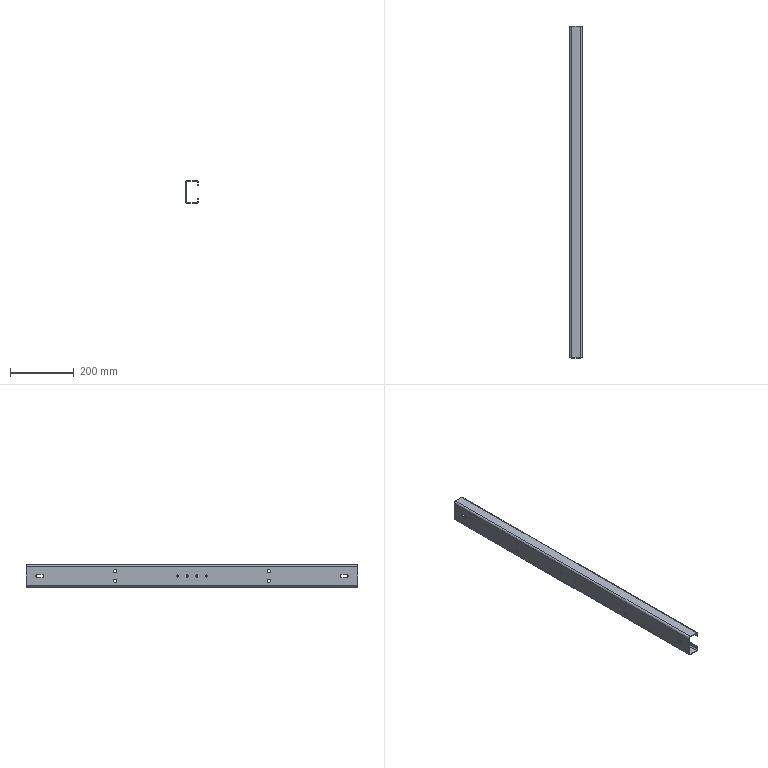Part | SolidWorks | features FlatPattern 1, ICE 1, SMBaseFlange 1, SheetMetal 1 | 1 solid | 62 faces | box 40 x 1038 x 70 mm | volume 337187 mm3 | plane 34 | cylinder 28 | commonest cylinder face diameters 11 x12 7 x8 8 x4 12 x4